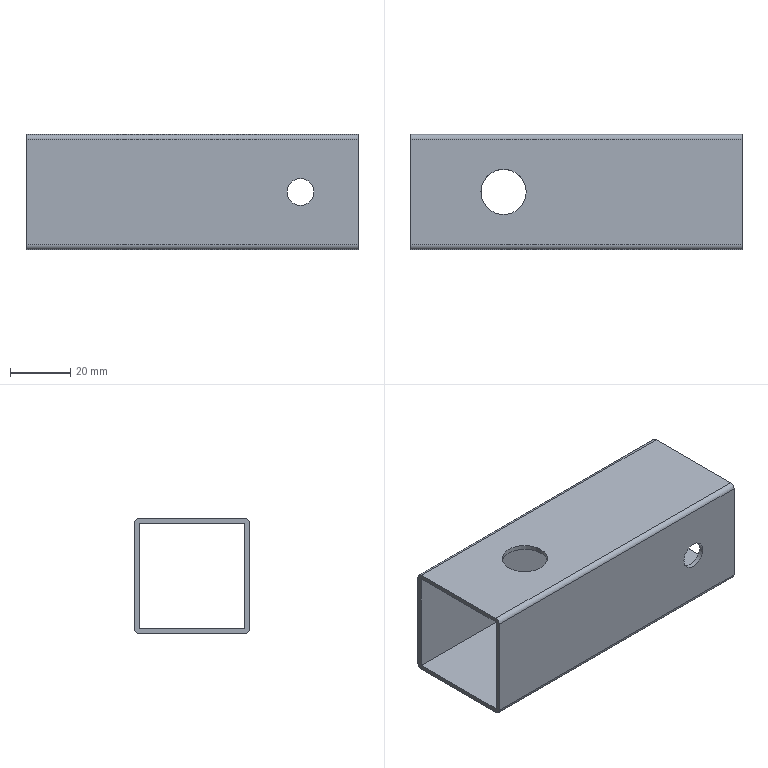Part | NX | features BREP 1 | 1 solid | 22 faces | box 109.982 x 38.1 x 38.1 mm | volume 23178 mm3 | cylinder 12 | plane 10 | commonest cylinder face diameters 3.175 x4 8.89 x4 14.986 x4
STEP:
#1=CARTESIAN_POINT('',(-54.991,19.05,-17.462));
#2=VERTEX_POINT('',#1);
#3=CARTESIAN_POINT('',(-54.991,19.05,17.462));
#4=VERTEX_POINT('',#3);
#5=CARTESIAN_POINT('',(-54.991,19.05,-17.462));
#6=DIRECTION('',(0.,0.,1.));
#7=VECTOR('',#6,1000.);
#8=LINE('',#5,#7);
#9=EDGE_CURVE('',#2,#4,#8,.T.);
#10=ORIENTED_EDGE('',*,*,#9,.F.);
#11=CARTESIAN_POINT('',(-54.991,17.462,-19.05));
#12=VERTEX_POINT('',#11);
#13=CARTESIAN_POINT('',(-54.991,17.462,-17.462));
#14=DIRECTION('',(-1.,0.,0.));
#15=DIRECTION('',(0.,1.,0.));
#16=AXIS2_PLACEMENT_3D('',#13,#14,#15);
#17=CIRCLE('',#16,1.587);
#18=EDGE_CURVE('',#2,#12,#17,.T.);
#19=ORIENTED_EDGE('',*,*,#18,.T.);
#20=CARTESIAN_POINT('',(-54.991,-17.462,-19.05));
#21=VERTEX_POINT('',#20);
#22=CARTESIAN_POINT('',(-54.991,-17.462,-19.05));
#23=DIRECTION('',(0.,1.,0.));
#24=VECTOR('',#23,1000.);
#25=LINE('',#22,#24);
#26=EDGE_CURVE('',#21,#12,#25,.T.);
#27=ORIENTED_EDGE('',*,*,#26,.F.);
#28=CARTESIAN_POINT('',(-54.991,-19.05,-17.462));
#29=VERTEX_POINT('',#28);
#30=CARTESIAN_POINT('',(-54.991,-17.462,-17.462));
#31=DIRECTION('',(-1.,0.,0.));
#32=DIRECTION('',(0.,0.,-1.));
#33=AXIS2_PLACEMENT_3D('',#30,#31,#32);
#34=CIRCLE('',#33,1.587);
#35=EDGE_CURVE('',#21,#29,#34,.T.);
#36=ORIENTED_EDGE('',*,*,#35,.T.);
#37=CARTESIAN_POINT('',(-54.991,-19.05,17.462));
#38=VERTEX_POINT('',#37);
#39=CARTESIAN_POINT('',(-54.991,-19.05,17.462));
#40=DIRECTION('',(0.,0.,-1.));
#41=VECTOR('',#40,1000.);
#42=LINE('',#39,#41);
#43=EDGE_CURVE('',#38,#29,#42,.T.);
#44=ORIENTED_EDGE('',*,*,#43,.F.);
#45=CARTESIAN_POINT('',(-54.991,-17.462,19.05));
#46=VERTEX_POINT('',#45);
#47=CARTESIAN_POINT('',(-54.991,-17.462,17.462));
#48=DIRECTION('',(-1.,0.,0.));
#49=DIRECTION('',(0.,-1.,0.));
#50=AXIS2_PLACEMENT_3D('',#47,#48,#49);
#51=CIRCLE('',#50,1.587);
#52=EDGE_CURVE('',#38,#46,#51,.T.);
#53=ORIENTED_EDGE('',*,*,#52,.T.);
#54=CARTESIAN_POINT('',(-54.991,17.462,19.05));
#55=VERTEX_POINT('',#54);
#56=CARTESIAN_POINT('',(-54.991,17.462,19.05));
#57=DIRECTION('',(0.,-1.,0.));
#58=VECTOR('',#57,1000.);
#59=LINE('',#56,#58);
#60=EDGE_CURVE('',#55,#46,#59,.T.);
#61=ORIENTED_EDGE('',*,*,#60,.F.);
#62=CARTESIAN_POINT('',(-54.991,17.462,17.462));
#63=DIRECTION('',(-1.,0.,0.));
#64=DIRECTION('',(0.,0.,1.));
#65=AXIS2_PLACEMENT_3D('',#62,#63,#64);
#66=CIRCLE('',#65,1.587);
#67=EDGE_CURVE('',#55,#4,#66,.T.);
#68=ORIENTED_EDGE('',*,*,#67,.T.);
#69=EDGE_LOOP('',(#10,#19,#27,#36,#44,#53,#61,#68));
#70=FACE_BOUND('',#69,.T.);
#71=CARTESIAN_POINT('',(-54.991,17.551,17.551));
#72=VERTEX_POINT('',#71);
#73=CARTESIAN_POINT('',(-54.991,17.551,-17.551));
#74=VERTEX_POINT('',#73);
#75=CARTESIAN_POINT('',(-54.991,17.551,17.551));
#76=DIRECTION('',(0.,0.,-1.));
#77=VECTOR('',#76,1000.);
#78=LINE('',#75,#77);
#79=EDGE_CURVE('',#72,#74,#78,.T.);
#80=ORIENTED_EDGE('',*,*,#79,.F.);
#81=CARTESIAN_POINT('',(-54.991,-17.551,17.551));
#82=VERTEX_POINT('',#81);
#83=CARTESIAN_POINT('',(-54.991,-17.551,17.551));
#84=DIRECTION('',(0.,1.,0.));
#85=VECTOR('',#84,1000.);
#86=LINE('',#83,#85);
#87=EDGE_CURVE('',#82,#72,#86,.T.);
#88=ORIENTED_EDGE('',*,*,#87,.F.);
#89=CARTESIAN_POINT('',(-54.991,-17.551,-17.551));
#90=VERTEX_POINT('',#89);
#91=CARTESIAN_POINT('',(-54.991,-17.551,-17.551));
#92=DIRECTION('',(0.,0.,1.));
#93=VECTOR('',#92,1000.);
#94=LINE('',#91,#93);
#95=EDGE_CURVE('',#90,#82,#94,.T.);
#96=ORIENTED_EDGE('',*,*,#95,.F.);
#97=CARTESIAN_POINT('',(-54.991,17.551,-17.551));
#98=DIRECTION('',(0.,-1.,0.));
#99=VECTOR('',#98,1000.);
#100=LINE('',#97,#99);
#101=EDGE_CURVE('',#74,#90,#100,.T.);
#102=ORIENTED_EDGE('',*,*,#101,.F.);
#103=EDGE_LOOP('',(#80,#88,#96,#102));
#104=FACE_BOUND('',#103,.T.);
#105=CARTESIAN_POINT('',(-54.991,0.,0.));
#106=DIRECTION('',(1.,0.,0.));
#107=DIRECTION('',(0.,1.,0.));
#108=AXIS2_PLACEMENT_3D('',#105,#106,#107);
#109=PLANE('',#108);
#110=ADVANCED_FACE('',(#70,#104),#109,.F.);
#111=CARTESIAN_POINT('',(54.991,-17.551,-17.551));
#112=VERTEX_POINT('',#111);
#113=CARTESIAN_POINT('',(-54.991,-17.551,-17.551));
#114=DIRECTION('',(1.,0.,0.));
#115=VECTOR('',#114,1000.);
#116=LINE('',#113,#115);
#117=EDGE_CURVE('',#90,#112,#116,.T.);
#118=ORIENTED_EDGE('',*,*,#117,.T.);
#119=CARTESIAN_POINT('',(54.991,17.551,-17.551));
#120=VERTEX_POINT('',#119);
#121=CARTESIAN_POINT('',(54.991,17.551,-17.551));
#122=DIRECTION('',(0.,-1.,0.));
#123=VECTOR('',#122,1000.);
#124=LINE('',#121,#123);
#125=EDGE_CURVE('',#120,#112,#124,.T.);
#126=ORIENTED_EDGE('',*,*,#125,.F.);
#127=CARTESIAN_POINT('',(-54.991,17.551,-17.551));
#128=DIRECTION('',(1.,0.,0.));
#129=VECTOR('',#128,1000.);
#130=LINE('',#127,#129);
#131=EDGE_CURVE('',#74,#120,#130,.T.);
#132=ORIENTED_EDGE('',*,*,#131,.F.);
#133=ORIENTED_EDGE('',*,*,#101,.T.);
#134=EDGE_LOOP('',(#118,#126,#132,#133));
#135=FACE_BOUND('',#134,.T.);
#136=CARTESIAN_POINT('',(-31.496,0.,-17.551));
#137=VERTEX_POINT('',#136);
#138=CARTESIAN_POINT('',(-16.51,0.,-17.551));
#139=VERTEX_POINT('',#138);
#140=CARTESIAN_POINT('',(-24.003,0.,-17.551));
#141=DIRECTION('',(0.,0.,1.));
#142=DIRECTION('',(-1.,0.,0.));
#143=AXIS2_PLACEMENT_3D('',#140,#141,#142);
#144=CIRCLE('',#143,7.493);
#145=EDGE_CURVE('',#137,#139,#144,.T.);
#146=ORIENTED_EDGE('',*,*,#145,.F.);
#147=CARTESIAN_POINT('',(-24.003,0.,-17.551));
#148=DIRECTION('',(0.,0.,1.));
#149=DIRECTION('',(1.,0.,0.));
#150=AXIS2_PLACEMENT_3D('',#147,#148,#149);
#151=CIRCLE('',#150,7.493);
#152=EDGE_CURVE('',#139,#137,#151,.T.);
#153=ORIENTED_EDGE('',*,*,#152,.F.);
#154=EDGE_LOOP('',(#146,#153));
#155=FACE_BOUND('',#154,.T.);
#156=CARTESIAN_POINT('',(-54.991,17.551,-17.551));
#157=DIRECTION('',(0.,0.,1.));
#158=DIRECTION('',(1.,0.,0.));
#159=AXIS2_PLACEMENT_3D('',#156,#157,#158);
#160=PLANE('',#159);
#161=ADVANCED_FACE('',(#135,#155),#160,.T.);
#162=ORIENTED_EDGE('',*,*,#131,.T.);
#163=CARTESIAN_POINT('',(54.991,17.551,17.551));
#164=VERTEX_POINT('',#163);
#165=CARTESIAN_POINT('',(54.991,17.551,17.551));
#166=DIRECTION('',(0.,0.,-1.));
#167=VECTOR('',#166,1000.);
#168=LINE('',#165,#167);
#169=EDGE_CURVE('',#164,#120,#168,.T.);
#170=ORIENTED_EDGE('',*,*,#169,.F.);
#171=CARTESIAN_POINT('',(-54.991,17.551,17.551));
#172=DIRECTION('',(1.,0.,0.));
#173=VECTOR('',#172,1000.);
#174=LINE('',#171,#173);
#175=EDGE_CURVE('',#72,#164,#174,.T.);
#176=ORIENTED_EDGE('',*,*,#175,.F.);
#177=ORIENTED_EDGE('',*,*,#79,.T.);
#178=EDGE_LOOP('',(#162,#170,#176,#177));
#179=FACE_BOUND('',#178,.T.);
#180=CARTESIAN_POINT('',(31.496,17.551,0.));
#181=VERTEX_POINT('',#180);
#182=CARTESIAN_POINT('',(40.386,17.551,0.));
#183=VERTEX_POINT('',#182);
#184=CARTESIAN_POINT('',(35.941,17.551,0.));
#185=DIRECTION('',(0.,1.,0.));
#186=DIRECTION('',(-1.,0.,0.));
#187=AXIS2_PLACEMENT_3D('',#184,#185,#186);
#188=CIRCLE('',#187,4.445);
#189=EDGE_CURVE('',#181,#183,#188,.T.);
#190=ORIENTED_EDGE('',*,*,#189,.T.);
#191=CARTESIAN_POINT('',(35.941,17.551,0.));
#192=DIRECTION('',(0.,1.,0.));
#193=DIRECTION('',(1.,0.,0.));
#194=AXIS2_PLACEMENT_3D('',#191,#192,#193);
#195=CIRCLE('',#194,4.445);
#196=EDGE_CURVE('',#183,#181,#195,.T.);
#197=ORIENTED_EDGE('',*,*,#196,.T.);
#198=EDGE_LOOP('',(#190,#197));
#199=FACE_BOUND('',#198,.T.);
#200=CARTESIAN_POINT('',(-54.991,17.551,17.551));
#201=DIRECTION('',(0.,-1.,0.));
#202=DIRECTION('',(0.,0.,-1.));
#203=AXIS2_PLACEMENT_3D('',#200,#201,#202);
#204=PLANE('',#203);
#205=ADVANCED_FACE('',(#179,#199),#204,.T.);
#206=ORIENTED_EDGE('',*,*,#175,.T.);
#207=CARTESIAN_POINT('',(54.991,-17.551,17.551));
#208=VERTEX_POINT('',#207);
#209=CARTESIAN_POINT('',(54.991,-17.551,17.551));
#210=DIRECTION('',(0.,1.,0.));
#211=VECTOR('',#210,1000.);
#212=LINE('',#209,#211);
#213=EDGE_CURVE('',#208,#164,#212,.T.);
#214=ORIENTED_EDGE('',*,*,#213,.F.);
#215=CARTESIAN_POINT('',(-54.991,-17.551,17.551));
#216=DIRECTION('',(1.,0.,0.));
#217=VECTOR('',#216,1000.);
#218=LINE('',#215,#217);
#219=EDGE_CURVE('',#82,#208,#218,.T.);
#220=ORIENTED_EDGE('',*,*,#219,.F.);
#221=ORIENTED_EDGE('',*,*,#87,.T.);
#222=EDGE_LOOP('',(#206,#214,#220,#221));
#223=FACE_BOUND('',#222,.T.);
#224=CARTESIAN_POINT('',(-31.496,0.,17.551));
#225=VERTEX_POINT('',#224);
#226=CARTESIAN_POINT('',(-16.51,0.,17.551));
#227=VERTEX_POINT('',#226);
#228=CARTESIAN_POINT('',(-24.003,0.,17.551));
#229=DIRECTION('',(0.,0.,1.));
#230=DIRECTION('',(-1.,0.,0.));
#231=AXIS2_PLACEMENT_3D('',#228,#229,#230);
#232=CIRCLE('',#231,7.493);
#233=EDGE_CURVE('',#225,#227,#232,.T.);
#234=ORIENTED_EDGE('',*,*,#233,.T.);
#235=CARTESIAN_POINT('',(-24.003,0.,17.551));
#236=DIRECTION('',(0.,0.,1.));
#237=DIRECTION('',(1.,0.,0.));
#238=AXIS2_PLACEMENT_3D('',#235,#236,#237);
#239=CIRCLE('',#238,7.493);
#240=EDGE_CURVE('',#227,#225,#239,.T.);
#241=ORIENTED_EDGE('',*,*,#240,.T.);
#242=EDGE_LOOP('',(#234,#241));
#243=FACE_BOUND('',#242,.T.);
#244=CARTESIAN_POINT('',(-54.991,-17.551,17.551));
#245=DIRECTION('',(0.,0.,-1.));
#246=DIRECTION('',(0.,-1.,0.));
#247=AXIS2_PLACEMENT_3D('',#244,#245,#246);
#248=PLANE('',#247);
#249=ADVANCED_FACE('',(#223,#243),#248,.T.);
#250=ORIENTED_EDGE('',*,*,#219,.T.);
#251=CARTESIAN_POINT('',(54.991,-17.551,-17.551));
#252=DIRECTION('',(0.,0.,1.));
#253=VECTOR('',#252,1000.);
#254=LINE('',#251,#253);
#255=EDGE_CURVE('',#112,#208,#254,.T.);
#256=ORIENTED_EDGE('',*,*,#255,.F.);
#257=ORIENTED_EDGE('',*,*,#117,.F.);
#258=ORIENTED_EDGE('',*,*,#95,.T.);
#259=EDGE_LOOP('',(#250,#256,#257,#258));
#260=FACE_BOUND('',#259,.T.);
#261=CARTESIAN_POINT('',(31.496,-17.551,0.));
#262=VERTEX_POINT('',#261);
#263=CARTESIAN_POINT('',(40.386,-17.551,0.));
#264=VERTEX_POINT('',#263);
#265=CARTESIAN_POINT('',(35.941,-17.551,0.));
#266=DIRECTION('',(0.,1.,0.));
#267=DIRECTION('',(-1.,0.,0.));
#268=AXIS2_PLACEMENT_3D('',#265,#266,#267);
#269=CIRCLE('',#268,4.445);
#270=EDGE_CURVE('',#262,#264,#269,.T.);
#271=ORIENTED_EDGE('',*,*,#270,.F.);
#272=CARTESIAN_POINT('',(35.941,-17.551,0.));
#273=DIRECTION('',(0.,1.,0.));
#274=DIRECTION('',(1.,0.,0.));
#275=AXIS2_PLACEMENT_3D('',#272,#273,#274);
#276=CIRCLE('',#275,4.445);
#277=EDGE_CURVE('',#264,#262,#276,.T.);
#278=ORIENTED_EDGE('',*,*,#277,.F.);
#279=EDGE_LOOP('',(#271,#278));
#280=FACE_BOUND('',#279,.T.);
#281=CARTESIAN_POINT('',(-54.991,-17.551,-17.551));
#282=DIRECTION('',(0.,1.,0.));
#283=DIRECTION('',(1.,0.,0.));
#284=AXIS2_PLACEMENT_3D('',#281,#282,#283);
#285=PLANE('',#284);
#286=ADVANCED_FACE('',(#260,#280),#285,.T.);
#287=CARTESIAN_POINT('',(54.991,17.462,19.05));
#288=VERTEX_POINT('',#287);
#289=CARTESIAN_POINT('',(54.991,-17.462,19.05));
#290=VERTEX_POINT('',#289);
#291=CARTESIAN_POINT('',(54.991,17.462,19.05));
#292=DIRECTION('',(0.,-1.,0.));
#293=VECTOR('',#292,1000.);
#294=LINE('',#291,#293);
#295=EDGE_CURVE('',#288,#290,#294,.T.);
#296=ORIENTED_EDGE('',*,*,#295,.T.);
#297=CARTESIAN_POINT('',(54.991,-19.05,17.462));
#298=VERTEX_POINT('',#297);
#299=CARTESIAN_POINT('',(54.991,-17.462,17.462));
#300=DIRECTION('',(1.,0.,0.));
#301=DIRECTION('',(0.,0.,1.));
#302=AXIS2_PLACEMENT_3D('',#299,#300,#301);
#303=CIRCLE('',#302,1.587);
#304=EDGE_CURVE('',#290,#298,#303,.T.);
#305=ORIENTED_EDGE('',*,*,#304,.T.);
#306=CARTESIAN_POINT('',(54.991,-19.05,-17.462));
#307=VERTEX_POINT('',#306);
#308=CARTESIAN_POINT('',(54.991,-19.05,17.462));
#309=DIRECTION('',(0.,0.,-1.));
#310=VECTOR('',#309,1000.);
#311=LINE('',#308,#310);
#312=EDGE_CURVE('',#298,#307,#311,.T.);
#313=ORIENTED_EDGE('',*,*,#312,.T.);
#314=CARTESIAN_POINT('',(54.991,-17.462,-19.05));
#315=VERTEX_POINT('',#314);
#316=CARTESIAN_POINT('',(54.991,-17.462,-17.462));
#317=DIRECTION('',(1.,0.,0.));
#318=DIRECTION('',(0.,-1.,0.));
#319=AXIS2_PLACEMENT_3D('',#316,#317,#318);
#320=CIRCLE('',#319,1.587);
#321=EDGE_CURVE('',#307,#315,#320,.T.);
#322=ORIENTED_EDGE('',*,*,#321,.T.);
#323=CARTESIAN_POINT('',(54.991,17.462,-19.05));
#324=VERTEX_POINT('',#323);
#325=CARTESIAN_POINT('',(54.991,-17.462,-19.05));
#326=DIRECTION('',(0.,1.,0.));
#327=VECTOR('',#326,1000.);
#328=LINE('',#325,#327);
#329=EDGE_CURVE('',#315,#324,#328,.T.);
#330=ORIENTED_EDGE('',*,*,#329,.T.);
#331=CARTESIAN_POINT('',(54.991,19.05,-17.462));
#332=VERTEX_POINT('',#331);
#333=CARTESIAN_POINT('',(54.991,17.462,-17.462));
#334=DIRECTION('',(1.,0.,0.));
#335=DIRECTION('',(0.,0.,-1.));
#336=AXIS2_PLACEMENT_3D('',#333,#334,#335);
#337=CIRCLE('',#336,1.587);
#338=EDGE_CURVE('',#324,#332,#337,.T.);
#339=ORIENTED_EDGE('',*,*,#338,.T.);
#340=CARTESIAN_POINT('',(54.991,19.05,17.462));
#341=VERTEX_POINT('',#340);
#342=CARTESIAN_POINT('',(54.991,19.05,-17.462));
#343=DIRECTION('',(0.,0.,1.));
#344=VECTOR('',#343,1000.);
#345=LINE('',#342,#344);
#346=EDGE_CURVE('',#332,#341,#345,.T.);
#347=ORIENTED_EDGE('',*,*,#346,.T.);
#348=CARTESIAN_POINT('',(54.991,17.462,17.462));
#349=DIRECTION('',(1.,0.,0.));
#350=DIRECTION('',(0.,1.,0.));
#351=AXIS2_PLACEMENT_3D('',#348,#349,#350);
#352=CIRCLE('',#351,1.587);
#353=EDGE_CURVE('',#341,#288,#352,.T.);
#354=ORIENTED_EDGE('',*,*,#353,.T.);
#355=EDGE_LOOP('',(#296,#305,#313,#322,#330,#339,#347,#354));
#356=FACE_BOUND('',#355,.T.);
#357=ORIENTED_EDGE('',*,*,#255,.T.);
#358=ORIENTED_EDGE('',*,*,#213,.T.);
#359=ORIENTED_EDGE('',*,*,#169,.T.);
#360=ORIENTED_EDGE('',*,*,#125,.T.);
#361=EDGE_LOOP('',(#357,#358,#359,#360));
#362=FACE_BOUND('',#361,.T.);
#363=CARTESIAN_POINT('',(54.991,0.,0.));
#364=DIRECTION('',(1.,0.,0.));
#365=DIRECTION('',(0.,1.,0.));
#366=AXIS2_PLACEMENT_3D('',#363,#364,#365);
#367=PLANE('',#366);
#368=ADVANCED_FACE('',(#356,#362),#367,.T.);
#369=ORIENTED_EDGE('',*,*,#353,.F.);
#370=CARTESIAN_POINT('',(54.991,19.05,17.462));
#371=DIRECTION('',(-1.,0.,0.));
#372=VECTOR('',#371,1000.);
#373=LINE('',#370,#372);
#374=EDGE_CURVE('',#341,#4,#373,.T.);
#375=ORIENTED_EDGE('',*,*,#374,.T.);
#376=ORIENTED_EDGE('',*,*,#67,.F.);
#377=CARTESIAN_POINT('',(54.991,17.462,19.05));
#378=DIRECTION('',(-1.,0.,0.));
#379=VECTOR('',#378,1000.);
#380=LINE('',#377,#379);
#381=EDGE_CURVE('',#288,#55,#380,.T.);
#382=ORIENTED_EDGE('',*,*,#381,.F.);
#383=EDGE_LOOP('',(#369,#375,#376,#382));
#384=FACE_BOUND('',#383,.T.);
#385=CARTESIAN_POINT('',(55.183,17.462,17.462));
#386=DIRECTION('',(-1.,0.,0.));
#387=DIRECTION('',(0.,0.,1.));
#388=AXIS2_PLACEMENT_3D('',#385,#386,#387);
#389=CYLINDRICAL_SURFACE('',#388,1.587);
#390=ADVANCED_FACE('',(#384),#389,.T.);
#391=ORIENTED_EDGE('',*,*,#60,.T.);
#392=CARTESIAN_POINT('',(54.991,-17.462,19.05));
#393=DIRECTION('',(-1.,0.,0.));
#394=VECTOR('',#393,1000.);
#395=LINE('',#392,#394);
#396=EDGE_CURVE('',#290,#46,#395,.T.);
#397=ORIENTED_EDGE('',*,*,#396,.F.);
#398=ORIENTED_EDGE('',*,*,#295,.F.);
#399=ORIENTED_EDGE('',*,*,#381,.T.);
#400=EDGE_LOOP('',(#391,#397,#398,#399));
#401=FACE_BOUND('',#400,.T.);
#402=CARTESIAN_POINT('',(-31.496,0.,19.05));
#403=VERTEX_POINT('',#402);
#404=CARTESIAN_POINT('',(-16.51,0.,19.05));
#405=VERTEX_POINT('',#404);
#406=CARTESIAN_POINT('',(-24.003,0.,19.05));
#407=DIRECTION('',(0.,0.,1.));
#408=DIRECTION('',(-1.,0.,0.));
#409=AXIS2_PLACEMENT_3D('',#406,#407,#408);
#410=CIRCLE('',#409,7.493);
#411=EDGE_CURVE('',#403,#405,#410,.T.);
#412=ORIENTED_EDGE('',*,*,#411,.F.);
#413=CARTESIAN_POINT('',(-24.003,0.,19.05));
#414=DIRECTION('',(0.,0.,1.));
#415=DIRECTION('',(1.,0.,0.));
#416=AXIS2_PLACEMENT_3D('',#413,#414,#415);
#417=CIRCLE('',#416,7.493);
#418=EDGE_CURVE('',#405,#403,#417,.T.);
#419=ORIENTED_EDGE('',*,*,#418,.F.);
#420=EDGE_LOOP('',(#412,#419));
#421=FACE_BOUND('',#420,.T.);
#422=CARTESIAN_POINT('',(-54.991,19.05,19.05));
#423=DIRECTION('',(0.,0.,1.));
#424=DIRECTION('',(1.,0.,0.));
#425=AXIS2_PLACEMENT_3D('',#422,#423,#424);
#426=PLANE('',#425);
#427=ADVANCED_FACE('',(#401,#421),#426,.T.);
#428=ORIENTED_EDGE('',*,*,#304,.F.);
#429=ORIENTED_EDGE('',*,*,#396,.T.);
#430=ORIENTED_EDGE('',*,*,#52,.F.);
#431=CARTESIAN_POINT('',(54.991,-19.05,17.462));
#432=DIRECTION('',(-1.,0.,0.));
#433=VECTOR('',#432,1000.);
#434=LINE('',#431,#433);
#435=EDGE_CURVE('',#298,#38,#434,.T.);
#436=ORIENTED_EDGE('',*,*,#435,.F.);
#437=EDGE_LOOP('',(#428,#429,#430,#436));
#438=FACE_BOUND('',#437,.T.);
#439=CARTESIAN_POINT('',(55.183,-17.462,17.462));
#440=DIRECTION('',(-1.,0.,0.));
#441=DIRECTION('',(0.,-1.,0.));
#442=AXIS2_PLACEMENT_3D('',#439,#440,#441);
#443=CYLINDRICAL_SURFACE('',#442,1.587);
#444=ADVANCED_FACE('',(#438),#443,.T.);
#445=ORIENTED_EDGE('',*,*,#43,.T.);
#446=CARTESIAN_POINT('',(54.991,-19.05,-17.462));
#447=DIRECTION('',(-1.,0.,0.));
#448=VECTOR('',#447,1000.);
#449=LINE('',#446,#448);
#450=EDGE_CURVE('',#307,#29,#449,.T.);
#451=ORIENTED_EDGE('',*,*,#450,.F.);
#452=ORIENTED_EDGE('',*,*,#312,.F.);
#453=ORIENTED_EDGE('',*,*,#435,.T.);
#454=EDGE_LOOP('',(#445,#451,#452,#453));
#455=FACE_BOUND('',#454,.T.);
#456=CARTESIAN_POINT('',(31.496,-19.05,0.));
#457=VERTEX_POINT('',#456);
#458=CARTESIAN_POINT('',(40.386,-19.05,0.));
#459=VERTEX_POINT('',#458);
#460=CARTESIAN_POINT('',(35.941,-19.05,0.));
#461=DIRECTION('',(0.,1.,0.));
#462=DIRECTION('',(-1.,0.,0.));
#463=AXIS2_PLACEMENT_3D('',#460,#461,#462);
#464=CIRCLE('',#463,4.445);
#465=EDGE_CURVE('',#457,#459,#464,.T.);
#466=ORIENTED_EDGE('',*,*,#465,.T.);
#467=CARTESIAN_POINT('',(35.941,-19.05,0.));
#468=DIRECTION('',(0.,1.,0.));
#469=DIRECTION('',(1.,0.,0.));
#470=AXIS2_PLACEMENT_3D('',#467,#468,#469);
#471=CIRCLE('',#470,4.445);
#472=EDGE_CURVE('',#459,#457,#471,.T.);
#473=ORIENTED_EDGE('',*,*,#472,.T.);
#474=EDGE_LOOP('',(#466,#473));
#475=FACE_BOUND('',#474,.T.);
#476=CARTESIAN_POINT('',(-54.991,-19.05,19.05));
#477=DIRECTION('',(0.,-1.,0.));
#478=DIRECTION('',(0.,0.,-1.));
#479=AXIS2_PLACEMENT_3D('',#476,#477,#478);
#480=PLANE('',#479);
#481=ADVANCED_FACE('',(#455,#475),#480,.T.);
#482=ORIENTED_EDGE('',*,*,#321,.F.);
#483=ORIENTED_EDGE('',*,*,#450,.T.);
#484=ORIENTED_EDGE('',*,*,#35,.F.);
#485=CARTESIAN_POINT('',(54.991,-17.462,-19.05));
#486=DIRECTION('',(-1.,0.,0.));
#487=VECTOR('',#486,1000.);
#488=LINE('',#485,#487);
#489=EDGE_CURVE('',#315,#21,#488,.T.);
#490=ORIENTED_EDGE('',*,*,#489,.F.);
#491=EDGE_LOOP('',(#482,#483,#484,#490));
#492=FACE_BOUND('',#491,.T.);
#493=CARTESIAN_POINT('',(55.183,-17.462,-17.462));
#494=DIRECTION('',(-1.,0.,0.));
#495=DIRECTION('',(0.,0.,-1.));
#496=AXIS2_PLACEMENT_3D('',#493,#494,#495);
#497=CYLINDRICAL_SURFACE('',#496,1.587);
#498=ADVANCED_FACE('',(#492),#497,.T.);
#499=ORIENTED_EDGE('',*,*,#329,.F.);
#500=ORIENTED_EDGE('',*,*,#489,.T.);
#501=ORIENTED_EDGE('',*,*,#26,.T.);
#502=CARTESIAN_POINT('',(54.991,17.462,-19.05));
#503=DIRECTION('',(-1.,0.,0.));
#504=VECTOR('',#503,1000.);
#505=LINE('',#502,#504);
#506=EDGE_CURVE('',#324,#12,#505,.T.);
#507=ORIENTED_EDGE('',*,*,#506,.F.);
#508=EDGE_LOOP('',(#499,#500,#501,#507));
#509=FACE_BOUND('',#508,.T.);
#510=CARTESIAN_POINT('',(-31.496,0.,-19.05));
#511=VERTEX_POINT('',#510);
#512=CARTESIAN_POINT('',(-16.51,0.,-19.05));
#513=VERTEX_POINT('',#512);
#514=CARTESIAN_POINT('',(-24.003,0.,-19.05));
#515=DIRECTION('',(0.,0.,1.));
#516=DIRECTION('',(-1.,0.,0.));
#517=AXIS2_PLACEMENT_3D('',#514,#515,#516);
#518=CIRCLE('',#517,7.493);
#519=EDGE_CURVE('',#511,#513,#518,.T.);
#520=ORIENTED_EDGE('',*,*,#519,.T.);
#521=CARTESIAN_POINT('',(-24.003,0.,-19.05));
#522=DIRECTION('',(0.,0.,1.));
#523=DIRECTION('',(1.,0.,0.));
#524=AXIS2_PLACEMENT_3D('',#521,#522,#523);
#525=CIRCLE('',#524,7.493);
#526=EDGE_CURVE('',#513,#511,#525,.T.);
#527=ORIENTED_EDGE('',*,*,#526,.T.);
#528=EDGE_LOOP('',(#520,#527));
#529=FACE_BOUND('',#528,.T.);
#530=CARTESIAN_POINT('',(-54.991,-19.05,-19.05));
#531=DIRECTION('',(0.,0.,-1.));
#532=DIRECTION('',(0.,-1.,0.));
#533=AXIS2_PLACEMENT_3D('',#530,#531,#532);
#534=PLANE('',#533);
#535=ADVANCED_FACE('',(#509,#529),#534,.T.);
#536=ORIENTED_EDGE('',*,*,#338,.F.);
#537=ORIENTED_EDGE('',*,*,#506,.T.);
#538=ORIENTED_EDGE('',*,*,#18,.F.);
#539=CARTESIAN_POINT('',(54.991,19.05,-17.462));
#540=DIRECTION('',(-1.,0.,0.));
#541=VECTOR('',#540,1000.);
#542=LINE('',#539,#541);
#543=EDGE_CURVE('',#332,#2,#542,.T.);
#544=ORIENTED_EDGE('',*,*,#543,.F.);
#545=EDGE_LOOP('',(#536,#537,#538,#544));
#546=FACE_BOUND('',#545,.T.);
#547=CARTESIAN_POINT('',(55.183,17.462,-17.462));
#548=DIRECTION('',(-1.,0.,0.));
#549=DIRECTION('',(0.,1.,0.));
#550=AXIS2_PLACEMENT_3D('',#547,#548,#549);
#551=CYLINDRICAL_SURFACE('',#550,1.587);
#552=ADVANCED_FACE('',(#546),#551,.T.);
#553=ORIENTED_EDGE('',*,*,#346,.F.);
#554=ORIENTED_EDGE('',*,*,#543,.T.);
#555=ORIENTED_EDGE('',*,*,#9,.T.);
#556=ORIENTED_EDGE('',*,*,#374,.F.);
#557=EDGE_LOOP('',(#553,#554,#555,#556));
#558=FACE_BOUND('',#557,.T.);
#559=CARTESIAN_POINT('',(31.496,19.05,0.));
#560=VERTEX_POINT('',#559);
#561=CARTESIAN_POINT('',(40.386,19.05,0.));
#562=VERTEX_POINT('',#561);
#563=CARTESIAN_POINT('',(35.941,19.05,0.));
#564=DIRECTION('',(0.,1.,0.));
#565=DIRECTION('',(-1.,0.,0.));
#566=AXIS2_PLACEMENT_3D('',#563,#564,#565);
#567=CIRCLE('',#566,4.445);
#568=EDGE_CURVE('',#560,#562,#567,.T.);
#569=ORIENTED_EDGE('',*,*,#568,.F.);
#570=CARTESIAN_POINT('',(35.941,19.05,0.));
#571=DIRECTION('',(0.,1.,0.));
#572=DIRECTION('',(1.,0.,0.));
#573=AXIS2_PLACEMENT_3D('',#570,#571,#572);
#574=CIRCLE('',#573,4.445);
#575=EDGE_CURVE('',#562,#560,#574,.T.);
#576=ORIENTED_EDGE('',*,*,#575,.F.);
#577=EDGE_LOOP('',(#569,#576));
#578=FACE_BOUND('',#577,.T.);
#579=CARTESIAN_POINT('',(-54.991,19.05,-19.05));
#580=DIRECTION('',(0.,1.,0.));
#581=DIRECTION('',(1.,0.,0.));
#582=AXIS2_PLACEMENT_3D('',#579,#580,#581);
#583=PLANE('',#582);
#584=ADVANCED_FACE('',(#558,#578),#583,.T.);
#585=CARTESIAN_POINT('',(31.496,19.05,0.));
#586=DIRECTION('',(0.,-1.,0.));
#587=VECTOR('',#586,1000.);
#588=LINE('',#585,#587);
#589=EDGE_CURVE('',#560,#181,#588,.T.);
#590=ORIENTED_EDGE('',*,*,#589,.T.);
#591=ORIENTED_EDGE('',*,*,#196,.F.);
#592=CARTESIAN_POINT('',(40.386,19.05,0.));
#593=DIRECTION('',(0.,-1.,0.));
#594=VECTOR('',#593,1000.);
#595=LINE('',#592,#594);
#596=EDGE_CURVE('',#562,#183,#595,.T.);
#597=ORIENTED_EDGE('',*,*,#596,.F.);
#598=ORIENTED_EDGE('',*,*,#575,.T.);
#599=EDGE_LOOP('',(#590,#591,#597,#598));
#600=FACE_BOUND('',#599,.T.);
#601=CARTESIAN_POINT('',(35.941,22.86,0.));
#602=DIRECTION('',(0.,1.,0.));
#603=DIRECTION('',(1.,0.,0.));
#604=AXIS2_PLACEMENT_3D('',#601,#602,#603);
#605=CYLINDRICAL_SURFACE('',#604,4.445);
#606=ADVANCED_FACE('',(#600),#605,.F.);
#607=CARTESIAN_POINT('',(40.386,-17.551,0.));
#608=DIRECTION('',(0.,-1.,0.));
#609=VECTOR('',#608,1000.);
#610=LINE('',#607,#609);
#611=EDGE_CURVE('',#459,#264,#610,.F.);
#612=ORIENTED_EDGE('',*,*,#611,.T.);
#613=ORIENTED_EDGE('',*,*,#277,.T.);
#614=CARTESIAN_POINT('',(31.496,-17.551,0.));
#615=DIRECTION('',(0.,-1.,0.));
#616=VECTOR('',#615,1000.);
#617=LINE('',#614,#616);
#618=EDGE_CURVE('',#457,#262,#617,.F.);
#619=ORIENTED_EDGE('',*,*,#618,.F.);
#620=ORIENTED_EDGE('',*,*,#472,.F.);
#621=EDGE_LOOP('',(#612,#613,#619,#620));
#622=FACE_BOUND('',#621,.T.);
#623=CARTESIAN_POINT('',(35.941,22.86,0.));
#624=DIRECTION('',(0.,1.,0.));
#625=DIRECTION('',(1.,0.,0.));
#626=AXIS2_PLACEMENT_3D('',#623,#624,#625);
#627=CYLINDRICAL_SURFACE('',#626,4.445);
#628=ADVANCED_FACE('',(#622),#627,.F.);
#629=ORIENTED_EDGE('',*,*,#596,.T.);
#630=ORIENTED_EDGE('',*,*,#189,.F.);
#631=ORIENTED_EDGE('',*,*,#589,.F.);
#632=ORIENTED_EDGE('',*,*,#568,.T.);
#633=EDGE_LOOP('',(#629,#630,#631,#632));
#634=FACE_BOUND('',#633,.T.);
#635=CARTESIAN_POINT('',(35.941,22.86,0.));
#636=DIRECTION('',(0.,1.,0.));
#637=DIRECTION('',(1.,0.,0.));
#638=AXIS2_PLACEMENT_3D('',#635,#636,#637);
#639=CYLINDRICAL_SURFACE('',#638,4.445);
#640=ADVANCED_FACE('',(#634),#639,.F.);
#641=ORIENTED_EDGE('',*,*,#618,.T.);
#642=ORIENTED_EDGE('',*,*,#270,.T.);
#643=ORIENTED_EDGE('',*,*,#611,.F.);
#644=ORIENTED_EDGE('',*,*,#465,.F.);
#645=EDGE_LOOP('',(#641,#642,#643,#644));
#646=FACE_BOUND('',#645,.T.);
#647=CARTESIAN_POINT('',(35.941,22.86,0.));
#648=DIRECTION('',(0.,1.,0.));
#649=DIRECTION('',(1.,0.,0.));
#650=AXIS2_PLACEMENT_3D('',#647,#648,#649);
#651=CYLINDRICAL_SURFACE('',#650,4.445);
#652=ADVANCED_FACE('',(#646),#651,.F.);
#653=CARTESIAN_POINT('',(-31.496,0.,19.05));
#654=DIRECTION('',(0.,0.,-1.));
#655=VECTOR('',#654,1000.);
#656=LINE('',#653,#655);
#657=EDGE_CURVE('',#403,#225,#656,.T.);
#658=ORIENTED_EDGE('',*,*,#657,.T.);
#659=ORIENTED_EDGE('',*,*,#240,.F.);
#660=CARTESIAN_POINT('',(-16.51,0.,19.05));
#661=DIRECTION('',(0.,0.,-1.));
#662=VECTOR('',#661,1000.);
#663=LINE('',#660,#662);
#664=EDGE_CURVE('',#405,#227,#663,.T.);
#665=ORIENTED_EDGE('',*,*,#664,.F.);
#666=ORIENTED_EDGE('',*,*,#418,.T.);
#667=EDGE_LOOP('',(#658,#659,#665,#666));
#668=FACE_BOUND('',#667,.T.);
#669=CARTESIAN_POINT('',(-24.003,0.,22.86));
#670=DIRECTION('',(0.,0.,1.));
#671=DIRECTION('',(1.,0.,0.));
#672=AXIS2_PLACEMENT_3D('',#669,#670,#671);
#673=CYLINDRICAL_SURFACE('',#672,7.493);
#674=ADVANCED_FACE('',(#668),#673,.F.);
#675=CARTESIAN_POINT('',(-16.51,0.,-17.551));
#676=DIRECTION('',(0.,0.,-1.));
#677=VECTOR('',#676,1000.);
#678=LINE('',#675,#677);
#679=EDGE_CURVE('',#513,#139,#678,.F.);
#680=ORIENTED_EDGE('',*,*,#679,.T.);
#681=ORIENTED_EDGE('',*,*,#152,.T.);
#682=CARTESIAN_POINT('',(-31.496,0.,-17.551));
#683=DIRECTION('',(0.,0.,-1.));
#684=VECTOR('',#683,1000.);
#685=LINE('',#682,#684);
#686=EDGE_CURVE('',#511,#137,#685,.F.);
#687=ORIENTED_EDGE('',*,*,#686,.F.);
#688=ORIENTED_EDGE('',*,*,#526,.F.);
#689=EDGE_LOOP('',(#680,#681,#687,#688));
#690=FACE_BOUND('',#689,.T.);
#691=CARTESIAN_POINT('',(-24.003,0.,22.86));
#692=DIRECTION('',(0.,0.,1.));
#693=DIRECTION('',(1.,0.,0.));
#694=AXIS2_PLACEMENT_3D('',#691,#692,#693);
#695=CYLINDRICAL_SURFACE('',#694,7.493);
#696=ADVANCED_FACE('',(#690),#695,.F.);
#697=ORIENTED_EDGE('',*,*,#664,.T.);
#698=ORIENTED_EDGE('',*,*,#233,.F.);
#699=ORIENTED_EDGE('',*,*,#657,.F.);
#700=ORIENTED_EDGE('',*,*,#411,.T.);
#701=EDGE_LOOP('',(#697,#698,#699,#700));
#702=FACE_BOUND('',#701,.T.);
#703=CARTESIAN_POINT('',(-24.003,0.,22.86));
#704=DIRECTION('',(0.,0.,1.));
#705=DIRECTION('',(1.,0.,0.));
#706=AXIS2_PLACEMENT_3D('',#703,#704,#705);
#707=CYLINDRICAL_SURFACE('',#706,7.493);
#708=ADVANCED_FACE('',(#702),#707,.F.);
#709=ORIENTED_EDGE('',*,*,#686,.T.);
#710=ORIENTED_EDGE('',*,*,#145,.T.);
#711=ORIENTED_EDGE('',*,*,#679,.F.);
#712=ORIENTED_EDGE('',*,*,#519,.F.);
#713=EDGE_LOOP('',(#709,#710,#711,#712));
#714=FACE_BOUND('',#713,.T.);
#715=CARTESIAN_POINT('',(-24.003,0.,22.86));
#716=DIRECTION('',(0.,0.,1.));
#717=DIRECTION('',(1.,0.,0.));
#718=AXIS2_PLACEMENT_3D('',#715,#716,#717);
#719=CYLINDRICAL_SURFACE('',#718,7.493);
#720=ADVANCED_FACE('',(#714),#719,.F.);
#721=CLOSED_SHELL('',(#110,#161,#205,#249,#286,#368,#390,#427,#444,#481,#498,#535,#552,#584,#606,#628,#640,#652,#674,#696,#708,#720));
#722=MANIFOLD_SOLID_BREP('',#721);
#723=(LENGTH_UNIT()NAMED_UNIT(*)SI_UNIT(.MILLI.,.METRE.));
#724=UNCERTAINTY_MEASURE_WITH_UNIT(LENGTH_MEASURE(0.00001),#723,'','');
#725=(NAMED_UNIT(*)PLANE_ANGLE_UNIT()SI_UNIT($,.RADIAN.));
#726=(NAMED_UNIT(*)SI_UNIT($,.STERADIAN.)SOLID_ANGLE_UNIT());
#727=(GEOMETRIC_REPRESENTATION_CONTEXT(3)GLOBAL_UNCERTAINTY_ASSIGNED_CONTEXT((#724))GLOBAL_UNIT_ASSIGNED_CONTEXT((#723,#725,#726))REPRESENTATION_CONTEXT('',''));
#728=ADVANCED_BREP_SHAPE_REPRESENTATION('',(#722),#727);